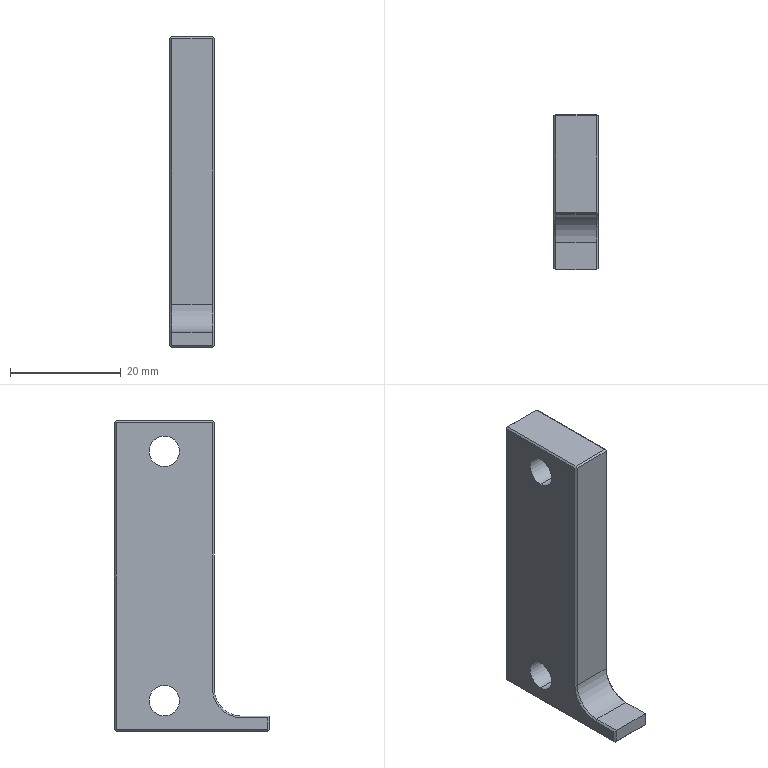Part | NX | 1 solid | 31 faces | box 8 x 28 x 56 mm | volume 7927 mm3 | plane 24 | cylinder 5 | cone 2 | commonest cylinder face diameters 5.5 x4 10 x1
STEP:
#1=CARTESIAN_POINT('',(2319.8,254.1,-75.2));
#2=VERTEX_POINT('',#1);
#3=CARTESIAN_POINT('',(2327.2,254.1,-75.2));
#4=VERTEX_POINT('',#3);
#5=CARTESIAN_POINT('',(2323.5,254.1,-75.2));
#6=DIRECTION('',(1.,0.,0.));
#7=VECTOR('',#6,1000.);
#8=LINE('',#5,#7);
#9=EDGE_CURVE('',#2,#4,#8,.T.);
#10=ORIENTED_EDGE('',*,*,#9,.T.);
#11=CARTESIAN_POINT('',(2327.2,226.7,-75.2));
#12=VERTEX_POINT('',#11);
#13=CARTESIAN_POINT('',(2327.2,240.4,-75.2));
#14=DIRECTION('',(0.,1.,0.));
#15=VECTOR('',#14,1000.);
#16=LINE('',#13,#15);
#17=EDGE_CURVE('',#12,#4,#16,.T.);
#18=ORIENTED_EDGE('',*,*,#17,.F.);
#19=CARTESIAN_POINT('',(2319.8,226.7,-75.2));
#20=VERTEX_POINT('',#19);
#21=CARTESIAN_POINT('',(2323.5,226.7,-75.2));
#22=DIRECTION('',(-1.,0.,0.));
#23=VECTOR('',#22,1000.);
#24=LINE('',#21,#23);
#25=EDGE_CURVE('',#12,#20,#24,.T.);
#26=ORIENTED_EDGE('',*,*,#25,.T.);
#27=CARTESIAN_POINT('',(2319.8,240.4,-75.2));
#28=DIRECTION('',(0.,-1.,0.));
#29=VECTOR('',#28,1000.);
#30=LINE('',#27,#29);
#31=EDGE_CURVE('',#2,#20,#30,.T.);
#32=ORIENTED_EDGE('',*,*,#31,.F.);
#33=EDGE_LOOP('',(#10,#18,#26,#32));
#34=FACE_BOUND('',#33,.T.);
#35=CARTESIAN_POINT('',(2321.5,254.4,-75.2));
#36=DIRECTION('',(0.,0.,-1.));
#37=DIRECTION('',(-1.,0.,0.));
#38=AXIS2_PLACEMENT_3D('',#35,#36,#37);
#39=PLANE('',#38);
#40=ADVANCED_FACE('',(#34),#39,.T.);
#41=CARTESIAN_POINT('',(2319.8,254.4,-19.5));
#42=VERTEX_POINT('',#41);
#43=CARTESIAN_POINT('',(2327.2,254.4,-19.5));
#44=VERTEX_POINT('',#43);
#45=CARTESIAN_POINT('',(2323.5,254.4,-19.5));
#46=DIRECTION('',(1.,0.,0.));
#47=VECTOR('',#46,1000.);
#48=LINE('',#45,#47);
#49=EDGE_CURVE('',#42,#44,#48,.T.);
#50=ORIENTED_EDGE('',*,*,#49,.T.);
#51=CARTESIAN_POINT('',(2327.2,254.4,-74.9));
#52=VERTEX_POINT('',#51);
#53=CARTESIAN_POINT('',(2327.2,254.4,-47.2));
#54=DIRECTION('',(0.,0.,1.));
#55=VECTOR('',#54,1000.);
#56=LINE('',#53,#55);
#57=EDGE_CURVE('',#52,#44,#56,.T.);
#58=ORIENTED_EDGE('',*,*,#57,.F.);
#59=CARTESIAN_POINT('',(2319.8,254.4,-74.9));
#60=VERTEX_POINT('',#59);
#61=CARTESIAN_POINT('',(2323.5,254.4,-74.9));
#62=DIRECTION('',(1.,0.,0.));
#63=VECTOR('',#62,1000.);
#64=LINE('',#61,#63);
#65=EDGE_CURVE('',#60,#52,#64,.T.);
#66=ORIENTED_EDGE('',*,*,#65,.F.);
#67=CARTESIAN_POINT('',(2319.8,254.4,-47.2));
#68=DIRECTION('',(0.,0.,-1.));
#69=VECTOR('',#68,1000.);
#70=LINE('',#67,#69);
#71=EDGE_CURVE('',#42,#60,#70,.T.);
#72=ORIENTED_EDGE('',*,*,#71,.F.);
#73=EDGE_LOOP('',(#50,#58,#66,#72));
#74=FACE_BOUND('',#73,.T.);
#75=CARTESIAN_POINT('',(2321.5,254.4,-19.2));
#76=DIRECTION('',(0.,1.,0.));
#77=DIRECTION('',(1.,0.,0.));
#78=AXIS2_PLACEMENT_3D('',#75,#76,#77);
#79=PLANE('',#78);
#80=ADVANCED_FACE('',(#74),#79,.T.);
#81=CARTESIAN_POINT('',(2319.8,236.7,-19.2));
#82=VERTEX_POINT('',#81);
#83=CARTESIAN_POINT('',(2327.2,236.7,-19.2));
#84=VERTEX_POINT('',#83);
#85=CARTESIAN_POINT('',(2323.5,236.7,-19.2));
#86=DIRECTION('',(1.,0.,0.));
#87=VECTOR('',#86,1000.);
#88=LINE('',#85,#87);
#89=EDGE_CURVE('',#82,#84,#88,.T.);
#90=ORIENTED_EDGE('',*,*,#89,.T.);
#91=CARTESIAN_POINT('',(2327.2,254.1,-19.2));
#92=VERTEX_POINT('',#91);
#93=CARTESIAN_POINT('',(2327.2,245.4,-19.2));
#94=DIRECTION('',(0.,-1.,0.));
#95=VECTOR('',#94,1000.);
#96=LINE('',#93,#95);
#97=EDGE_CURVE('',#92,#84,#96,.T.);
#98=ORIENTED_EDGE('',*,*,#97,.F.);
#99=CARTESIAN_POINT('',(2319.8,254.1,-19.2));
#100=VERTEX_POINT('',#99);
#101=CARTESIAN_POINT('',(2323.5,254.1,-19.2));
#102=DIRECTION('',(1.,0.,0.));
#103=VECTOR('',#102,1000.);
#104=LINE('',#101,#103);
#105=EDGE_CURVE('',#100,#92,#104,.T.);
#106=ORIENTED_EDGE('',*,*,#105,.F.);
#107=CARTESIAN_POINT('',(2319.8,245.4,-19.2));
#108=DIRECTION('',(0.,1.,0.));
#109=VECTOR('',#108,1000.);
#110=LINE('',#107,#109);
#111=EDGE_CURVE('',#82,#100,#110,.T.);
#112=ORIENTED_EDGE('',*,*,#111,.F.);
#113=EDGE_LOOP('',(#90,#98,#106,#112));
#114=FACE_BOUND('',#113,.T.);
#115=CARTESIAN_POINT('',(2321.5,236.4,-19.2));
#116=DIRECTION('',(0.,0.,1.));
#117=DIRECTION('',(1.,0.,0.));
#118=AXIS2_PLACEMENT_3D('',#115,#116,#117);
#119=PLANE('',#118);
#120=ADVANCED_FACE('',(#114),#119,.T.);
#121=CARTESIAN_POINT('',(2327.2,236.4,-67.5));
#122=VERTEX_POINT('',#121);
#123=CARTESIAN_POINT('',(2319.8,236.4,-67.5));
#124=VERTEX_POINT('',#123);
#125=CARTESIAN_POINT('',(2321.5,236.4,-67.5));
#126=DIRECTION('',(-1.,0.,0.));
#127=VECTOR('',#126,1000.);
#128=LINE('',#125,#127);
#129=EDGE_CURVE('',#122,#124,#128,.T.);
#130=ORIENTED_EDGE('',*,*,#129,.F.);
#131=CARTESIAN_POINT('',(2327.2,236.4,-19.5));
#132=VERTEX_POINT('',#131);
#133=CARTESIAN_POINT('',(2327.2,236.4,-43.35));
#134=DIRECTION('',(0.,0.,-1.));
#135=VECTOR('',#134,1000.);
#136=LINE('',#133,#135);
#137=EDGE_CURVE('',#132,#122,#136,.T.);
#138=ORIENTED_EDGE('',*,*,#137,.F.);
#139=CARTESIAN_POINT('',(2319.8,236.4,-19.5));
#140=VERTEX_POINT('',#139);
#141=CARTESIAN_POINT('',(2323.5,236.4,-19.5));
#142=DIRECTION('',(1.,0.,0.));
#143=VECTOR('',#142,1000.);
#144=LINE('',#141,#143);
#145=EDGE_CURVE('',#140,#132,#144,.T.);
#146=ORIENTED_EDGE('',*,*,#145,.F.);
#147=CARTESIAN_POINT('',(2319.8,236.4,-43.35));
#148=DIRECTION('',(0.,0.,1.));
#149=VECTOR('',#148,1000.);
#150=LINE('',#147,#149);
#151=EDGE_CURVE('',#124,#140,#150,.T.);
#152=ORIENTED_EDGE('',*,*,#151,.F.);
#153=EDGE_LOOP('',(#130,#138,#146,#152));
#154=FACE_BOUND('',#153,.T.);
#155=CARTESIAN_POINT('',(2321.5,236.4,-75.2));
#156=DIRECTION('',(0.,-1.,0.));
#157=DIRECTION('',(0.,0.,-1.));
#158=AXIS2_PLACEMENT_3D('',#155,#156,#157);
#159=PLANE('',#158);
#160=ADVANCED_FACE('',(#154),#159,.T.);
#161=CARTESIAN_POINT('',(2319.8,226.4,-72.5));
#162=VERTEX_POINT('',#161);
#163=CARTESIAN_POINT('',(2319.8,226.4,-74.9));
#164=VERTEX_POINT('',#163);
#165=CARTESIAN_POINT('',(2319.8,226.4,-73.85));
#166=DIRECTION('',(0.,0.,-1.));
#167=VECTOR('',#166,1000.);
#168=LINE('',#165,#167);
#169=EDGE_CURVE('',#162,#164,#168,.T.);
#170=ORIENTED_EDGE('',*,*,#169,.T.);
#171=CARTESIAN_POINT('',(2327.2,226.4,-74.9));
#172=VERTEX_POINT('',#171);
#173=CARTESIAN_POINT('',(2323.5,226.4,-74.9));
#174=DIRECTION('',(-1.,0.,0.));
#175=VECTOR('',#174,1000.);
#176=LINE('',#173,#175);
#177=EDGE_CURVE('',#172,#164,#176,.T.);
#178=ORIENTED_EDGE('',*,*,#177,.F.);
#179=CARTESIAN_POINT('',(2327.2,226.4,-72.5));
#180=VERTEX_POINT('',#179);
#181=CARTESIAN_POINT('',(2327.2,226.4,-73.85));
#182=DIRECTION('',(0.,0.,-1.));
#183=VECTOR('',#182,1000.);
#184=LINE('',#181,#183);
#185=EDGE_CURVE('',#180,#172,#184,.T.);
#186=ORIENTED_EDGE('',*,*,#185,.F.);
#187=CARTESIAN_POINT('',(2321.5,226.4,-72.5));
#188=DIRECTION('',(-1.,0.,0.));
#189=VECTOR('',#188,1000.);
#190=LINE('',#187,#189);
#191=EDGE_CURVE('',#180,#162,#190,.T.);
#192=ORIENTED_EDGE('',*,*,#191,.T.);
#193=EDGE_LOOP('',(#170,#178,#186,#192));
#194=FACE_BOUND('',#193,.T.);
#195=CARTESIAN_POINT('',(2325.077,226.4,-68.526));
#196=DIRECTION('',(0.,-1.,0.));
#197=DIRECTION('',(0.,0.,-1.));
#198=AXIS2_PLACEMENT_3D('',#195,#196,#197);
#199=PLANE('',#198);
#200=ADVANCED_FACE('',(#194),#199,.T.);
#201=CARTESIAN_POINT('',(2319.8,231.4,-72.5));
#202=VERTEX_POINT('',#201);
#203=CARTESIAN_POINT('',(2319.8,228.9,-72.5));
#204=DIRECTION('',(0.,-1.,0.));
#205=VECTOR('',#204,1000.);
#206=LINE('',#203,#205);
#207=EDGE_CURVE('',#202,#162,#206,.T.);
#208=ORIENTED_EDGE('',*,*,#207,.T.);
#209=ORIENTED_EDGE('',*,*,#191,.F.);
#210=CARTESIAN_POINT('',(2327.2,231.4,-72.5));
#211=VERTEX_POINT('',#210);
#212=CARTESIAN_POINT('',(2327.2,228.9,-72.5));
#213=DIRECTION('',(0.,-1.,0.));
#214=VECTOR('',#213,1000.);
#215=LINE('',#212,#214);
#216=EDGE_CURVE('',#211,#180,#215,.T.);
#217=ORIENTED_EDGE('',*,*,#216,.F.);
#218=CARTESIAN_POINT('',(2321.5,231.4,-72.5));
#219=DIRECTION('',(-1.,0.,0.));
#220=VECTOR('',#219,1000.);
#221=LINE('',#218,#220);
#222=EDGE_CURVE('',#211,#202,#221,.T.);
#223=ORIENTED_EDGE('',*,*,#222,.T.);
#224=EDGE_LOOP('',(#208,#209,#217,#223));
#225=FACE_BOUND('',#224,.T.);
#226=CARTESIAN_POINT('',(2321.5,236.4,-72.5));
#227=DIRECTION('',(0.,0.,1.));
#228=DIRECTION('',(1.,0.,0.));
#229=AXIS2_PLACEMENT_3D('',#226,#227,#228);
#230=PLANE('',#229);
#231=ADVANCED_FACE('',(#225),#230,.T.);
#232=CARTESIAN_POINT('',(2327.2,231.4,-67.5));
#233=DIRECTION('',(-1.,0.,0.));
#234=DIRECTION('',(0.,0.,-1.));
#235=AXIS2_PLACEMENT_3D('',#232,#233,#234);
#236=CIRCLE('',#235,5.);
#237=EDGE_CURVE('',#122,#211,#236,.T.);
#238=ORIENTED_EDGE('',*,*,#237,.F.);
#239=ORIENTED_EDGE('',*,*,#129,.T.);
#240=CARTESIAN_POINT('',(2319.8,231.4,-67.5));
#241=DIRECTION('',(-1.,0.,0.));
#242=DIRECTION('',(0.,0.,-1.));
#243=AXIS2_PLACEMENT_3D('',#240,#241,#242);
#244=CIRCLE('',#243,5.);
#245=EDGE_CURVE('',#124,#202,#244,.T.);
#246=ORIENTED_EDGE('',*,*,#245,.T.);
#247=ORIENTED_EDGE('',*,*,#222,.F.);
#248=EDGE_LOOP('',(#238,#239,#246,#247));
#249=FACE_BOUND('',#248,.T.);
#250=CARTESIAN_POINT('',(2321.5,231.4,-67.5));
#251=DIRECTION('',(-1.,0.,0.));
#252=DIRECTION('',(0.,0.,-1.));
#253=AXIS2_PLACEMENT_3D('',#250,#251,#252);
#254=CYLINDRICAL_SURFACE('',#253,5.);
#255=ADVANCED_FACE('',(#249),#254,.F.);
#256=ORIENTED_EDGE('',*,*,#9,.F.);
#257=CARTESIAN_POINT('',(2319.65,254.25,-75.05));
#258=VERTEX_POINT('',#257);
#259=CARTESIAN_POINT('',(2327.326,246.574,-82.726));
#260=DIRECTION('',(0.5774,-0.5774,-0.5774));
#261=VECTOR('',#260,1000.);
#262=LINE('',#259,#261);
#263=EDGE_CURVE('',#258,#2,#262,.T.);
#264=ORIENTED_EDGE('',*,*,#263,.F.);
#265=CARTESIAN_POINT('',(2321.5,256.1,-73.2));
#266=DIRECTION('',(0.5774,0.5774,0.5774));
#267=VECTOR('',#266,1000.);
#268=LINE('',#265,#267);
#269=EDGE_CURVE('',#258,#60,#268,.T.);
#270=ORIENTED_EDGE('',*,*,#269,.T.);
#271=ORIENTED_EDGE('',*,*,#65,.T.);
#272=CARTESIAN_POINT('',(2327.35,254.25,-75.05));
#273=VERTEX_POINT('',#272);
#274=CARTESIAN_POINT('',(2321.5,260.1,-69.2));
#275=DIRECTION('',(0.5774,-0.5774,-0.5774));
#276=VECTOR('',#275,1000.);
#277=LINE('',#274,#276);
#278=EDGE_CURVE('',#52,#273,#277,.T.);
#279=ORIENTED_EDGE('',*,*,#278,.T.);
#280=CARTESIAN_POINT('',(2319.674,246.574,-82.726));
#281=DIRECTION('',(-0.5774,-0.5774,-0.5774));
#282=VECTOR('',#281,1000.);
#283=LINE('',#280,#282);
#284=EDGE_CURVE('',#273,#4,#283,.T.);
#285=ORIENTED_EDGE('',*,*,#284,.T.);
#286=EDGE_LOOP('',(#256,#264,#270,#271,#279,#285));
#287=FACE_BOUND('',#286,.T.);
#288=CARTESIAN_POINT('',(2323.5,254.25,-75.05));
#289=DIRECTION('',(0.,0.7071,-0.7071));
#290=DIRECTION('',(-1.,0.,0.));
#291=AXIS2_PLACEMENT_3D('',#288,#289,#290);
#292=PLANE('',#291);
#293=ADVANCED_FACE('',(#287),#292,.T.);
#294=ORIENTED_EDGE('',*,*,#49,.F.);
#295=CARTESIAN_POINT('',(2319.65,254.25,-19.35));
#296=VERTEX_POINT('',#295);
#297=CARTESIAN_POINT('',(2345.565,280.165,-45.265));
#298=DIRECTION('',(0.5774,0.5774,-0.5774));
#299=VECTOR('',#298,1000.);
#300=LINE('',#297,#299);
#301=EDGE_CURVE('',#296,#42,#300,.T.);
#302=ORIENTED_EDGE('',*,*,#301,.F.);
#303=CARTESIAN_POINT('',(2293.735,280.165,-45.265));
#304=DIRECTION('',(0.5774,-0.5774,0.5774));
#305=VECTOR('',#304,1000.);
#306=LINE('',#303,#305);
#307=EDGE_CURVE('',#296,#100,#306,.T.);
#308=ORIENTED_EDGE('',*,*,#307,.T.);
#309=ORIENTED_EDGE('',*,*,#105,.T.);
#310=CARTESIAN_POINT('',(2327.35,254.25,-19.35));
#311=VERTEX_POINT('',#310);
#312=CARTESIAN_POINT('',(2353.265,280.165,-45.265));
#313=DIRECTION('',(0.5774,0.5774,-0.5774));
#314=VECTOR('',#313,1000.);
#315=LINE('',#312,#314);
#316=EDGE_CURVE('',#92,#311,#315,.T.);
#317=ORIENTED_EDGE('',*,*,#316,.T.);
#318=CARTESIAN_POINT('',(2301.435,280.165,-45.265));
#319=DIRECTION('',(0.5774,-0.5774,0.5774));
#320=VECTOR('',#319,1000.);
#321=LINE('',#318,#320);
#322=EDGE_CURVE('',#44,#311,#321,.T.);
#323=ORIENTED_EDGE('',*,*,#322,.F.);
#324=EDGE_LOOP('',(#294,#302,#308,#309,#317,#323));
#325=FACE_BOUND('',#324,.T.);
#326=CARTESIAN_POINT('',(2323.5,254.25,-19.35));
#327=DIRECTION('',(0.,0.7071,0.7071));
#328=DIRECTION('',(1.,0.,0.));
#329=AXIS2_PLACEMENT_3D('',#326,#327,#328);
#330=PLANE('',#329);
#331=ADVANCED_FACE('',(#325),#330,.T.);
#332=ORIENTED_EDGE('',*,*,#89,.F.);
#333=CARTESIAN_POINT('',(2319.65,236.55,-19.35));
#334=VERTEX_POINT('',#333);
#335=CARTESIAN_POINT('',(2293.735,210.635,-45.265));
#336=DIRECTION('',(0.5774,0.5774,0.5774));
#337=VECTOR('',#336,1000.);
#338=LINE('',#335,#337);
#339=EDGE_CURVE('',#334,#82,#338,.T.);
#340=ORIENTED_EDGE('',*,*,#339,.F.);
#341=CARTESIAN_POINT('',(2345.565,210.635,-45.265));
#342=DIRECTION('',(0.5774,-0.5774,-0.5774));
#343=VECTOR('',#342,1000.);
#344=LINE('',#341,#343);
#345=EDGE_CURVE('',#334,#140,#344,.T.);
#346=ORIENTED_EDGE('',*,*,#345,.T.);
#347=ORIENTED_EDGE('',*,*,#145,.T.);
#348=CARTESIAN_POINT('',(2327.35,236.55,-19.35));
#349=VERTEX_POINT('',#348);
#350=CARTESIAN_POINT('',(2301.435,210.635,-45.265));
#351=DIRECTION('',(0.5774,0.5774,0.5774));
#352=VECTOR('',#351,1000.);
#353=LINE('',#350,#352);
#354=EDGE_CURVE('',#132,#349,#353,.T.);
#355=ORIENTED_EDGE('',*,*,#354,.T.);
#356=CARTESIAN_POINT('',(2353.265,210.635,-45.265));
#357=DIRECTION('',(-0.5774,0.5774,0.5774));
#358=VECTOR('',#357,1000.);
#359=LINE('',#356,#358);
#360=EDGE_CURVE('',#349,#84,#359,.T.);
#361=ORIENTED_EDGE('',*,*,#360,.T.);
#362=EDGE_LOOP('',(#332,#340,#346,#347,#355,#361));
#363=FACE_BOUND('',#362,.T.);
#364=CARTESIAN_POINT('',(2323.5,236.55,-19.35));
#365=DIRECTION('',(0.,-0.7071,0.7071));
#366=DIRECTION('',(-1.,0.,0.));
#367=AXIS2_PLACEMENT_3D('',#364,#365,#366);
#368=PLANE('',#367);
#369=ADVANCED_FACE('',(#363),#368,.T.);
#370=ORIENTED_EDGE('',*,*,#245,.F.);
#371=CARTESIAN_POINT('',(2319.5,236.7,-67.5));
#372=VERTEX_POINT('',#371);
#373=CARTESIAN_POINT('',(2319.8,236.4,-67.5));
#374=DIRECTION('',(-0.7071,0.7071,0.));
#375=VECTOR('',#374,1000.);
#376=LINE('',#373,#375);
#377=EDGE_CURVE('',#124,#372,#376,.T.);
#378=ORIENTED_EDGE('',*,*,#377,.T.);
#379=CARTESIAN_POINT('',(2319.5,231.4,-72.8));
#380=VERTEX_POINT('',#379);
#381=CARTESIAN_POINT('',(2319.5,231.4,-67.5));
#382=DIRECTION('',(-1.,0.,0.));
#383=DIRECTION('',(0.,0.,-1.));
#384=AXIS2_PLACEMENT_3D('',#381,#382,#383);
#385=CIRCLE('',#384,5.3);
#386=EDGE_CURVE('',#372,#380,#385,.T.);
#387=ORIENTED_EDGE('',*,*,#386,.T.);
#388=CARTESIAN_POINT('',(2319.5,231.4,-72.8));
#389=DIRECTION('',(0.7071,0.,0.7071));
#390=VECTOR('',#389,1000.);
#391=LINE('',#388,#390);
#392=EDGE_CURVE('',#380,#202,#391,.T.);
#393=ORIENTED_EDGE('',*,*,#392,.T.);
#394=EDGE_LOOP('',(#370,#378,#387,#393));
#395=FACE_BOUND('',#394,.T.);
#396=CARTESIAN_POINT('',(2319.8,231.4,-67.5));
#397=DIRECTION('',(-1.,0.,0.));
#398=DIRECTION('',(0.,1.,0.));
#399=AXIS2_PLACEMENT_3D('',#396,#397,#398);
#400=CONICAL_SURFACE('',#399,5.,0.7854);
#401=ADVANCED_FACE('',(#395),#400,.F.);
#402=ORIENTED_EDGE('',*,*,#207,.F.);
#403=ORIENTED_EDGE('',*,*,#392,.F.);
#404=CARTESIAN_POINT('',(2319.5,226.7,-72.8));
#405=VERTEX_POINT('',#404);
#406=CARTESIAN_POINT('',(2319.5,228.9,-72.8));
#407=DIRECTION('',(0.,-1.,0.));
#408=VECTOR('',#407,1000.);
#409=LINE('',#406,#408);
#410=EDGE_CURVE('',#380,#405,#409,.T.);
#411=ORIENTED_EDGE('',*,*,#410,.T.);
#412=CARTESIAN_POINT('',(2299.626,246.574,-92.674));
#413=DIRECTION('',(-0.5774,0.5774,-0.5774));
#414=VECTOR('',#413,1000.);
#415=LINE('',#412,#414);
#416=EDGE_CURVE('',#162,#405,#415,.T.);
#417=ORIENTED_EDGE('',*,*,#416,.F.);
#418=EDGE_LOOP('',(#402,#403,#411,#417));
#419=FACE_BOUND('',#418,.T.);
#420=CARTESIAN_POINT('',(2319.65,228.9,-72.65));
#421=DIRECTION('',(-0.7071,0.,0.7071));
#422=DIRECTION('',(0.,1.,0.));
#423=AXIS2_PLACEMENT_3D('',#420,#421,#422);
#424=PLANE('',#423);
#425=ADVANCED_FACE('',(#419),#424,.T.);
#426=ORIENTED_EDGE('',*,*,#237,.T.);
#427=CARTESIAN_POINT('',(2327.5,231.4,-72.8));
#428=VERTEX_POINT('',#427);
#429=CARTESIAN_POINT('',(2327.2,231.4,-72.5));
#430=DIRECTION('',(0.7071,0.,-0.7071));
#431=VECTOR('',#430,1000.);
#432=LINE('',#429,#431);
#433=EDGE_CURVE('',#211,#428,#432,.T.);
#434=ORIENTED_EDGE('',*,*,#433,.T.);
#435=CARTESIAN_POINT('',(2327.5,236.7,-67.5));
#436=VERTEX_POINT('',#435);
#437=CARTESIAN_POINT('',(2327.5,231.4,-67.5));
#438=DIRECTION('',(-1.,0.,0.));
#439=DIRECTION('',(0.,0.,-1.));
#440=AXIS2_PLACEMENT_3D('',#437,#438,#439);
#441=CIRCLE('',#440,5.3);
#442=EDGE_CURVE('',#436,#428,#441,.T.);
#443=ORIENTED_EDGE('',*,*,#442,.F.);
#444=CARTESIAN_POINT('',(2327.2,236.4,-67.5));
#445=DIRECTION('',(0.7071,0.7071,0.));
#446=VECTOR('',#445,1000.);
#447=LINE('',#444,#446);
#448=EDGE_CURVE('',#122,#436,#447,.T.);
#449=ORIENTED_EDGE('',*,*,#448,.F.);
#450=EDGE_LOOP('',(#426,#434,#443,#449));
#451=FACE_BOUND('',#450,.T.);
#452=CARTESIAN_POINT('',(2327.2,231.4,-67.5));
#453=DIRECTION('',(1.,0.,0.));
#454=DIRECTION('',(0.,-1.,0.));
#455=AXIS2_PLACEMENT_3D('',#452,#453,#454);
#456=CONICAL_SURFACE('',#455,5.,0.7854);
#457=ADVANCED_FACE('',(#451),#456,.F.);
#458=ORIENTED_EDGE('',*,*,#177,.T.);
#459=CARTESIAN_POINT('',(2319.65,226.55,-75.05));
#460=VERTEX_POINT('',#459);
#461=CARTESIAN_POINT('',(2349.435,196.765,-45.265));
#462=DIRECTION('',(-0.5774,0.5774,-0.5774));
#463=VECTOR('',#462,1000.);
#464=LINE('',#461,#463);
#465=EDGE_CURVE('',#164,#460,#464,.T.);
#466=ORIENTED_EDGE('',*,*,#465,.T.);
#467=CARTESIAN_POINT('',(2289.865,196.765,-45.265));
#468=DIRECTION('',(0.5774,0.5774,-0.5774));
#469=VECTOR('',#468,1000.);
#470=LINE('',#467,#469);
#471=EDGE_CURVE('',#460,#20,#470,.T.);
#472=ORIENTED_EDGE('',*,*,#471,.T.);
#473=ORIENTED_EDGE('',*,*,#25,.F.);
#474=CARTESIAN_POINT('',(2327.35,226.55,-75.05));
#475=VERTEX_POINT('',#474);
#476=CARTESIAN_POINT('',(2357.135,196.765,-45.265));
#477=DIRECTION('',(0.5774,-0.5774,0.5774));
#478=VECTOR('',#477,1000.);
#479=LINE('',#476,#478);
#480=EDGE_CURVE('',#12,#475,#479,.T.);
#481=ORIENTED_EDGE('',*,*,#480,.T.);
#482=CARTESIAN_POINT('',(2297.565,196.765,-45.265));
#483=DIRECTION('',(0.5774,0.5774,-0.5774));
#484=VECTOR('',#483,1000.);
#485=LINE('',#482,#484);
#486=EDGE_CURVE('',#172,#475,#485,.T.);
#487=ORIENTED_EDGE('',*,*,#486,.F.);
#488=EDGE_LOOP('',(#458,#466,#472,#473,#481,#487));
#489=FACE_BOUND('',#488,.T.);
#490=CARTESIAN_POINT('',(2323.5,226.55,-75.05));
#491=DIRECTION('',(0.,0.7071,0.7071));
#492=DIRECTION('',(1.,0.,0.));
#493=AXIS2_PLACEMENT_3D('',#490,#491,#492);
#494=PLANE('',#493);
#495=ADVANCED_FACE('',(#489),#494,.F.);
#496=ORIENTED_EDGE('',*,*,#185,.T.);
#497=ORIENTED_EDGE('',*,*,#486,.T.);
#498=CARTESIAN_POINT('',(2327.5,226.7,-74.9));
#499=VERTEX_POINT('',#498);
#500=CARTESIAN_POINT('',(2357.135,256.335,-45.265));
#501=DIRECTION('',(-0.5774,-0.5774,-0.5774));
#502=VECTOR('',#501,1000.);
#503=LINE('',#500,#502);
#504=EDGE_CURVE('',#499,#475,#503,.T.);
#505=ORIENTED_EDGE('',*,*,#504,.F.);
#506=CARTESIAN_POINT('',(2327.5,226.7,-72.8));
#507=VERTEX_POINT('',#506);
#508=CARTESIAN_POINT('',(2327.5,226.7,-73.85));
#509=DIRECTION('',(0.,0.,-1.));
#510=VECTOR('',#509,1000.);
#511=LINE('',#508,#510);
#512=EDGE_CURVE('',#507,#499,#511,.T.);
#513=ORIENTED_EDGE('',*,*,#512,.F.);
#514=CARTESIAN_POINT('',(2299.965,199.165,-45.265));
#515=DIRECTION('',(0.5774,0.5774,-0.5774));
#516=VECTOR('',#515,1000.);
#517=LINE('',#514,#516);
#518=EDGE_CURVE('',#180,#507,#517,.T.);
#519=ORIENTED_EDGE('',*,*,#518,.F.);
#520=EDGE_LOOP('',(#496,#497,#505,#513,#519));
#521=FACE_BOUND('',#520,.T.);
#522=CARTESIAN_POINT('',(2327.35,226.55,-73.85));
#523=DIRECTION('',(-0.7071,0.7071,0.));
#524=DIRECTION('',(0.,0.,1.));
#525=AXIS2_PLACEMENT_3D('',#522,#523,#524);
#526=PLANE('',#525);
#527=ADVANCED_FACE('',(#521),#526,.F.);
#528=ORIENTED_EDGE('',*,*,#169,.F.);
#529=ORIENTED_EDGE('',*,*,#416,.T.);
#530=CARTESIAN_POINT('',(2319.5,226.7,-74.9));
#531=VERTEX_POINT('',#530);
#532=CARTESIAN_POINT('',(2319.5,226.7,-73.85));
#533=DIRECTION('',(0.,0.,-1.));
#534=VECTOR('',#533,1000.);
#535=LINE('',#532,#534);
#536=EDGE_CURVE('',#405,#531,#535,.T.);
#537=ORIENTED_EDGE('',*,*,#536,.T.);
#538=CARTESIAN_POINT('',(2299.626,246.574,-55.026));
#539=DIRECTION('',(0.5774,-0.5774,-0.5774));
#540=VECTOR('',#539,1000.);
#541=LINE('',#538,#540);
#542=EDGE_CURVE('',#531,#460,#541,.T.);
#543=ORIENTED_EDGE('',*,*,#542,.T.);
#544=ORIENTED_EDGE('',*,*,#465,.F.);
#545=EDGE_LOOP('',(#528,#529,#537,#543,#544));
#546=FACE_BOUND('',#545,.T.);
#547=CARTESIAN_POINT('',(2319.65,226.55,-73.85));
#548=DIRECTION('',(-0.7071,-0.7071,0.));
#549=DIRECTION('',(-0.7071,0.7071,0.));
#550=AXIS2_PLACEMENT_3D('',#547,#548,#549);
#551=PLANE('',#550);
#552=ADVANCED_FACE('',(#546),#551,.T.);
#553=CARTESIAN_POINT('',(2327.5,228.9,-72.8));
#554=DIRECTION('',(0.,-1.,0.));
#555=VECTOR('',#554,1000.);
#556=LINE('',#553,#555);
#557=EDGE_CURVE('',#428,#507,#556,.T.);
#558=ORIENTED_EDGE('',*,*,#557,.T.);
#559=ORIENTED_EDGE('',*,*,#512,.T.);
#560=CARTESIAN_POINT('',(2327.5,254.1,-74.9));
#561=VERTEX_POINT('',#560);
#562=CARTESIAN_POINT('',(2327.5,240.4,-74.9));
#563=DIRECTION('',(0.,1.,0.));
#564=VECTOR('',#563,1000.);
#565=LINE('',#562,#564);
#566=EDGE_CURVE('',#499,#561,#565,.T.);
#567=ORIENTED_EDGE('',*,*,#566,.T.);
#568=CARTESIAN_POINT('',(2327.5,254.1,-19.5));
#569=VERTEX_POINT('',#568);
#570=CARTESIAN_POINT('',(2327.5,254.1,-47.2));
#571=DIRECTION('',(0.,0.,1.));
#572=VECTOR('',#571,1000.);
#573=LINE('',#570,#572);
#574=EDGE_CURVE('',#561,#569,#573,.T.);
#575=ORIENTED_EDGE('',*,*,#574,.T.);
#576=CARTESIAN_POINT('',(2327.5,236.7,-19.5));
#577=VERTEX_POINT('',#576);
#578=CARTESIAN_POINT('',(2327.5,245.4,-19.5));
#579=DIRECTION('',(0.,-1.,0.));
#580=VECTOR('',#579,1000.);
#581=LINE('',#578,#580);
#582=EDGE_CURVE('',#569,#577,#581,.T.);
#583=ORIENTED_EDGE('',*,*,#582,.T.);
#584=CARTESIAN_POINT('',(2327.5,236.7,-43.35));
#585=DIRECTION('',(0.,0.,-1.));
#586=VECTOR('',#585,1000.);
#587=LINE('',#584,#586);
#588=EDGE_CURVE('',#577,#436,#587,.T.);
#589=ORIENTED_EDGE('',*,*,#588,.T.);
#590=ORIENTED_EDGE('',*,*,#442,.T.);
#591=EDGE_LOOP('',(#558,#559,#567,#575,#583,#589,#590));
#592=FACE_BOUND('',#591,.T.);
#593=CARTESIAN_POINT('',(2327.5,245.4,-72.45));
#594=VERTEX_POINT('',#593);
#595=CARTESIAN_POINT('',(2327.5,245.4,-66.95));
#596=VERTEX_POINT('',#595);
#597=CARTESIAN_POINT('',(2327.5,245.4,-69.7));
#598=DIRECTION('',(1.,0.,0.));
#599=DIRECTION('',(0.,0.,-1.));
#600=AXIS2_PLACEMENT_3D('',#597,#598,#599);
#601=CIRCLE('',#600,2.75);
#602=EDGE_CURVE('',#594,#596,#601,.T.);
#603=ORIENTED_EDGE('',*,*,#602,.F.);
#604=CARTESIAN_POINT('',(2327.5,245.4,-69.7));
#605=DIRECTION('',(1.,0.,0.));
#606=DIRECTION('',(0.,0.,-1.));
#607=AXIS2_PLACEMENT_3D('',#604,#605,#606);
#608=CIRCLE('',#607,2.75);
#609=EDGE_CURVE('',#596,#594,#608,.T.);
#610=ORIENTED_EDGE('',*,*,#609,.F.);
#611=EDGE_LOOP('',(#603,#610));
#612=FACE_BOUND('',#611,.T.);
#613=CARTESIAN_POINT('',(2327.5,245.4,-21.95));
#614=VERTEX_POINT('',#613);
#615=CARTESIAN_POINT('',(2327.5,245.4,-27.45));
#616=VERTEX_POINT('',#615);
#617=CARTESIAN_POINT('',(2327.5,245.4,-24.7));
#618=DIRECTION('',(1.,0.,0.));
#619=DIRECTION('',(0.,0.,-1.));
#620=AXIS2_PLACEMENT_3D('',#617,#618,#619);
#621=CIRCLE('',#620,2.75);
#622=EDGE_CURVE('',#614,#616,#621,.T.);
#623=ORIENTED_EDGE('',*,*,#622,.F.);
#624=CARTESIAN_POINT('',(2327.5,245.4,-24.7));
#625=DIRECTION('',(1.,0.,0.));
#626=DIRECTION('',(0.,0.,-1.));
#627=AXIS2_PLACEMENT_3D('',#624,#625,#626);
#628=CIRCLE('',#627,2.75);
#629=EDGE_CURVE('',#616,#614,#628,.T.);
#630=ORIENTED_EDGE('',*,*,#629,.F.);
#631=EDGE_LOOP('',(#623,#630));
#632=FACE_BOUND('',#631,.T.);
#633=CARTESIAN_POINT('',(2327.5,246.574,-45.265));
#634=DIRECTION('',(1.,0.,0.));
#635=DIRECTION('',(0.,1.,0.));
#636=AXIS2_PLACEMENT_3D('',#633,#634,#635);
#637=PLANE('',#636);
#638=ADVANCED_FACE('',(#592,#612,#632),#637,.T.);
#639=CARTESIAN_POINT('',(2319.5,245.4,-27.45));
#640=VERTEX_POINT('',#639);
#641=CARTESIAN_POINT('',(2319.5,245.4,-21.95));
#642=VERTEX_POINT('',#641);
#643=CARTESIAN_POINT('',(2319.5,245.4,-24.7));
#644=DIRECTION('',(1.,0.,0.));
#645=DIRECTION('',(0.,0.,-1.));
#646=AXIS2_PLACEMENT_3D('',#643,#644,#645);
#647=CIRCLE('',#646,2.75);
#648=EDGE_CURVE('',#640,#642,#647,.T.);
#649=ORIENTED_EDGE('',*,*,#648,.F.);
#650=CARTESIAN_POINT('',(2320.9,245.4,-27.45));
#651=DIRECTION('',(1.,0.,0.));
#652=VECTOR('',#651,1000.);
#653=LINE('',#650,#652);
#654=EDGE_CURVE('',#616,#640,#653,.F.);
#655=ORIENTED_EDGE('',*,*,#654,.F.);
#656=ORIENTED_EDGE('',*,*,#629,.T.);
#657=CARTESIAN_POINT('',(2320.9,245.4,-21.95));
#658=DIRECTION('',(1.,0.,0.));
#659=VECTOR('',#658,1000.);
#660=LINE('',#657,#659);
#661=EDGE_CURVE('',#614,#642,#660,.F.);
#662=ORIENTED_EDGE('',*,*,#661,.T.);
#663=EDGE_LOOP('',(#649,#655,#656,#662));
#664=FACE_BOUND('',#663,.T.);
#665=CARTESIAN_POINT('',(2320.9,245.4,-24.7));
#666=DIRECTION('',(1.,0.,0.));
#667=DIRECTION('',(0.,0.,-1.));
#668=AXIS2_PLACEMENT_3D('',#665,#666,#667);
#669=CYLINDRICAL_SURFACE('',#668,2.75);
#670=ADVANCED_FACE('',(#664),#669,.F.);
#671=ORIENTED_EDGE('',*,*,#602,.T.);
#672=CARTESIAN_POINT('',(2319.5,245.4,-66.95));
#673=VERTEX_POINT('',#672);
#674=CARTESIAN_POINT('',(2320.9,245.4,-66.95));
#675=DIRECTION('',(1.,0.,0.));
#676=VECTOR('',#675,1000.);
#677=LINE('',#674,#676);
#678=EDGE_CURVE('',#596,#673,#677,.F.);
#679=ORIENTED_EDGE('',*,*,#678,.T.);
#680=CARTESIAN_POINT('',(2319.5,245.4,-72.45));
#681=VERTEX_POINT('',#680);
#682=CARTESIAN_POINT('',(2319.5,245.4,-69.7));
#683=DIRECTION('',(1.,0.,0.));
#684=DIRECTION('',(0.,0.,-1.));
#685=AXIS2_PLACEMENT_3D('',#682,#683,#684);
#686=CIRCLE('',#685,2.75);
#687=EDGE_CURVE('',#681,#673,#686,.T.);
#688=ORIENTED_EDGE('',*,*,#687,.F.);
#689=CARTESIAN_POINT('',(2320.9,245.4,-72.45));
#690=DIRECTION('',(1.,0.,0.));
#691=VECTOR('',#690,1000.);
#692=LINE('',#689,#691);
#693=EDGE_CURVE('',#594,#681,#692,.F.);
#694=ORIENTED_EDGE('',*,*,#693,.F.);
#695=EDGE_LOOP('',(#671,#679,#688,#694));
#696=FACE_BOUND('',#695,.T.);
#697=CARTESIAN_POINT('',(2320.9,245.4,-69.7));
#698=DIRECTION('',(1.,0.,0.));
#699=DIRECTION('',(0.,0.,-1.));
#700=AXIS2_PLACEMENT_3D('',#697,#698,#699);
#701=CYLINDRICAL_SURFACE('',#700,2.75);
#702=ADVANCED_FACE('',(#696),#701,.F.);
#703=ORIENTED_EDGE('',*,*,#566,.F.);
#704=ORIENTED_EDGE('',*,*,#504,.T.);
#705=ORIENTED_EDGE('',*,*,#480,.F.);
#706=ORIENTED_EDGE('',*,*,#17,.T.);
#707=ORIENTED_EDGE('',*,*,#284,.F.);
#708=CARTESIAN_POINT('',(2357.135,224.465,-45.265));
#709=DIRECTION('',(0.5774,-0.5774,0.5774));
#710=VECTOR('',#709,1000.);
#711=LINE('',#708,#710);
#712=EDGE_CURVE('',#273,#561,#711,.T.);
#713=ORIENTED_EDGE('',*,*,#712,.T.);
#714=EDGE_LOOP('',(#703,#704,#705,#706,#707,#713));
#715=FACE_BOUND('',#714,.T.);
#716=CARTESIAN_POINT('',(2327.35,240.4,-75.05));
#717=DIRECTION('',(0.7071,0.,-0.7071));
#718=DIRECTION('',(0.,-1.,0.));
#719=AXIS2_PLACEMENT_3D('',#716,#717,#718);
#720=PLANE('',#719);
#721=ADVANCED_FACE('',(#715),#720,.T.);
#722=ORIENTED_EDGE('',*,*,#574,.F.);
#723=ORIENTED_EDGE('',*,*,#712,.F.);
#724=ORIENTED_EDGE('',*,*,#278,.F.);
#725=ORIENTED_EDGE('',*,*,#57,.T.);
#726=ORIENTED_EDGE('',*,*,#322,.T.);
#727=CARTESIAN_POINT('',(2353.265,228.335,-45.265));
#728=DIRECTION('',(0.5774,-0.5774,-0.5774));
#729=VECTOR('',#728,1000.);
#730=LINE('',#727,#729);
#731=EDGE_CURVE('',#311,#569,#730,.T.);
#732=ORIENTED_EDGE('',*,*,#731,.T.);
#733=EDGE_LOOP('',(#722,#723,#724,#725,#726,#732));
#734=FACE_BOUND('',#733,.T.);
#735=CARTESIAN_POINT('',(2327.35,254.25,-47.2));
#736=DIRECTION('',(0.7071,0.7071,0.));
#737=DIRECTION('',(0.,0.,-1.));
#738=AXIS2_PLACEMENT_3D('',#735,#736,#737);
#739=PLANE('',#738);
#740=ADVANCED_FACE('',(#734),#739,.T.);
#741=ORIENTED_EDGE('',*,*,#582,.F.);
#742=ORIENTED_EDGE('',*,*,#731,.F.);
#743=ORIENTED_EDGE('',*,*,#316,.F.);
#744=ORIENTED_EDGE('',*,*,#97,.T.);
#745=ORIENTED_EDGE('',*,*,#360,.F.);
#746=CARTESIAN_POINT('',(2353.265,262.465,-45.265));
#747=DIRECTION('',(0.5774,0.5774,-0.5774));
#748=VECTOR('',#747,1000.);
#749=LINE('',#746,#748);
#750=EDGE_CURVE('',#349,#577,#749,.T.);
#751=ORIENTED_EDGE('',*,*,#750,.T.);
#752=EDGE_LOOP('',(#741,#742,#743,#744,#745,#751));
#753=FACE_BOUND('',#752,.T.);
#754=CARTESIAN_POINT('',(2327.35,245.4,-19.35));
#755=DIRECTION('',(0.7071,0.,0.7071));
#756=DIRECTION('',(0.,-1.,0.));
#757=AXIS2_PLACEMENT_3D('',#754,#755,#756);
#758=PLANE('',#757);
#759=ADVANCED_FACE('',(#753),#758,.T.);
#760=ORIENTED_EDGE('',*,*,#588,.F.);
#761=ORIENTED_EDGE('',*,*,#750,.F.);
#762=ORIENTED_EDGE('',*,*,#354,.F.);
#763=ORIENTED_EDGE('',*,*,#137,.T.);
#764=ORIENTED_EDGE('',*,*,#448,.T.);
#765=EDGE_LOOP('',(#760,#761,#762,#763,#764));
#766=FACE_BOUND('',#765,.T.);
#767=CARTESIAN_POINT('',(2327.35,236.55,-43.35));
#768=DIRECTION('',(0.7071,-0.7071,0.));
#769=DIRECTION('',(0.,0.,-1.));
#770=AXIS2_PLACEMENT_3D('',#767,#768,#769);
#771=PLANE('',#770);
#772=ADVANCED_FACE('',(#766),#771,.T.);
#773=ORIENTED_EDGE('',*,*,#557,.F.);
#774=ORIENTED_EDGE('',*,*,#433,.F.);
#775=ORIENTED_EDGE('',*,*,#216,.T.);
#776=ORIENTED_EDGE('',*,*,#518,.T.);
#777=EDGE_LOOP('',(#773,#774,#775,#776));
#778=FACE_BOUND('',#777,.T.);
#779=CARTESIAN_POINT('',(2327.35,228.9,-72.65));
#780=DIRECTION('',(0.7071,0.,0.7071));
#781=DIRECTION('',(0.,-1.,0.));
#782=AXIS2_PLACEMENT_3D('',#779,#780,#781);
#783=PLANE('',#782);
#784=ADVANCED_FACE('',(#778),#783,.T.);
#785=CARTESIAN_POINT('',(2319.5,236.7,-19.5));
#786=VERTEX_POINT('',#785);
#787=CARTESIAN_POINT('',(2319.5,236.7,-43.35));
#788=DIRECTION('',(0.,0.,1.));
#789=VECTOR('',#788,1000.);
#790=LINE('',#787,#789);
#791=EDGE_CURVE('',#372,#786,#790,.T.);
#792=ORIENTED_EDGE('',*,*,#791,.F.);
#793=ORIENTED_EDGE('',*,*,#377,.F.);
#794=ORIENTED_EDGE('',*,*,#151,.T.);
#795=ORIENTED_EDGE('',*,*,#345,.F.);
#796=CARTESIAN_POINT('',(2293.735,262.465,-45.265));
#797=DIRECTION('',(0.5774,-0.5774,0.5774));
#798=VECTOR('',#797,1000.);
#799=LINE('',#796,#798);
#800=EDGE_CURVE('',#786,#334,#799,.T.);
#801=ORIENTED_EDGE('',*,*,#800,.F.);
#802=EDGE_LOOP('',(#792,#793,#794,#795,#801));
#803=FACE_BOUND('',#802,.T.);
#804=CARTESIAN_POINT('',(2319.65,236.55,-43.35));
#805=DIRECTION('',(-0.7071,-0.7071,0.));
#806=DIRECTION('',(-0.7071,0.7071,0.));
#807=AXIS2_PLACEMENT_3D('',#804,#805,#806);
#808=PLANE('',#807);
#809=ADVANCED_FACE('',(#803),#808,.T.);
#810=CARTESIAN_POINT('',(2319.5,254.1,-19.5));
#811=VERTEX_POINT('',#810);
#812=CARTESIAN_POINT('',(2319.5,245.4,-19.5));
#813=DIRECTION('',(0.,1.,0.));
#814=VECTOR('',#813,1000.);
#815=LINE('',#812,#814);
#816=EDGE_CURVE('',#786,#811,#815,.T.);
#817=ORIENTED_EDGE('',*,*,#816,.F.);
#818=ORIENTED_EDGE('',*,*,#800,.T.);
#819=ORIENTED_EDGE('',*,*,#339,.T.);
#820=ORIENTED_EDGE('',*,*,#111,.T.);
#821=ORIENTED_EDGE('',*,*,#307,.F.);
#822=CARTESIAN_POINT('',(2293.735,228.335,-45.265));
#823=DIRECTION('',(0.5774,0.5774,0.5774));
#824=VECTOR('',#823,1000.);
#825=LINE('',#822,#824);
#826=EDGE_CURVE('',#811,#296,#825,.T.);
#827=ORIENTED_EDGE('',*,*,#826,.F.);
#828=EDGE_LOOP('',(#817,#818,#819,#820,#821,#827));
#829=FACE_BOUND('',#828,.T.);
#830=CARTESIAN_POINT('',(2319.65,245.4,-19.35));
#831=DIRECTION('',(-0.7071,0.,0.7071));
#832=DIRECTION('',(0.,1.,0.));
#833=AXIS2_PLACEMENT_3D('',#830,#831,#832);
#834=PLANE('',#833);
#835=ADVANCED_FACE('',(#829),#834,.T.);
#836=ORIENTED_EDGE('',*,*,#791,.T.);
#837=ORIENTED_EDGE('',*,*,#816,.T.);
#838=CARTESIAN_POINT('',(2319.5,254.1,-74.9));
#839=VERTEX_POINT('',#838);
#840=CARTESIAN_POINT('',(2319.5,254.1,-47.2));
#841=DIRECTION('',(0.,0.,-1.));
#842=VECTOR('',#841,1000.);
#843=LINE('',#840,#842);
#844=EDGE_CURVE('',#811,#839,#843,.T.);
#845=ORIENTED_EDGE('',*,*,#844,.T.);
#846=CARTESIAN_POINT('',(2319.5,240.4,-74.9));
#847=DIRECTION('',(0.,-1.,0.));
#848=VECTOR('',#847,1000.);
#849=LINE('',#846,#848);
#850=EDGE_CURVE('',#839,#531,#849,.T.);
#851=ORIENTED_EDGE('',*,*,#850,.T.);
#852=ORIENTED_EDGE('',*,*,#536,.F.);
#853=ORIENTED_EDGE('',*,*,#410,.F.);
#854=ORIENTED_EDGE('',*,*,#386,.F.);
#855=EDGE_LOOP('',(#836,#837,#845,#851,#852,#853,#854));
#856=FACE_BOUND('',#855,.T.);
#857=ORIENTED_EDGE('',*,*,#648,.T.);
#858=CARTESIAN_POINT('',(2319.5,245.4,-24.7));
#859=DIRECTION('',(1.,0.,0.));
#860=DIRECTION('',(0.,0.,-1.));
#861=AXIS2_PLACEMENT_3D('',#858,#859,#860);
#862=CIRCLE('',#861,2.75);
#863=EDGE_CURVE('',#642,#640,#862,.T.);
#864=ORIENTED_EDGE('',*,*,#863,.T.);
#865=EDGE_LOOP('',(#857,#864));
#866=FACE_BOUND('',#865,.T.);
#867=ORIENTED_EDGE('',*,*,#687,.T.);
#868=CARTESIAN_POINT('',(2319.5,245.4,-69.7));
#869=DIRECTION('',(1.,0.,0.));
#870=DIRECTION('',(0.,0.,-1.));
#871=AXIS2_PLACEMENT_3D('',#868,#869,#870);
#872=CIRCLE('',#871,2.75);
#873=EDGE_CURVE('',#673,#681,#872,.T.);
#874=ORIENTED_EDGE('',*,*,#873,.T.);
#875=EDGE_LOOP('',(#867,#874));
#876=FACE_BOUND('',#875,.T.);
#877=CARTESIAN_POINT('',(2319.5,246.574,-45.265));
#878=DIRECTION('',(1.,0.,0.));
#879=DIRECTION('',(0.,1.,0.));
#880=AXIS2_PLACEMENT_3D('',#877,#878,#879);
#881=PLANE('',#880);
#882=ADVANCED_FACE('',(#856,#866,#876),#881,.F.);
#883=ORIENTED_EDGE('',*,*,#850,.F.);
#884=CARTESIAN_POINT('',(2289.865,224.465,-45.265));
#885=DIRECTION('',(0.5774,0.5774,-0.5774));
#886=VECTOR('',#885,1000.);
#887=LINE('',#884,#886);
#888=EDGE_CURVE('',#839,#258,#887,.T.);
#889=ORIENTED_EDGE('',*,*,#888,.T.);
#890=ORIENTED_EDGE('',*,*,#263,.T.);
#891=ORIENTED_EDGE('',*,*,#31,.T.);
#892=ORIENTED_EDGE('',*,*,#471,.F.);
#893=ORIENTED_EDGE('',*,*,#542,.F.);
#894=EDGE_LOOP('',(#883,#889,#890,#891,#892,#893));
#895=FACE_BOUND('',#894,.T.);
#896=CARTESIAN_POINT('',(2319.65,240.4,-75.05));
#897=DIRECTION('',(-0.7071,0.,-0.7071));
#898=DIRECTION('',(-0.7071,0.,0.7071));
#899=AXIS2_PLACEMENT_3D('',#896,#897,#898);
#900=PLANE('',#899);
#901=ADVANCED_FACE('',(#895),#900,.T.);
#902=ORIENTED_EDGE('',*,*,#844,.F.);
#903=ORIENTED_EDGE('',*,*,#826,.T.);
#904=ORIENTED_EDGE('',*,*,#301,.T.);
#905=ORIENTED_EDGE('',*,*,#71,.T.);
#906=ORIENTED_EDGE('',*,*,#269,.F.);
#907=ORIENTED_EDGE('',*,*,#888,.F.);
#908=EDGE_LOOP('',(#902,#903,#904,#905,#906,#907));
#909=FACE_BOUND('',#908,.T.);
#910=CARTESIAN_POINT('',(2319.65,254.25,-47.2));
#911=DIRECTION('',(-0.7071,0.7071,0.));
#912=DIRECTION('',(0.,0.,1.));
#913=AXIS2_PLACEMENT_3D('',#910,#911,#912);
#914=PLANE('',#913);
#915=ADVANCED_FACE('',(#909),#914,.T.);
#916=ORIENTED_EDGE('',*,*,#622,.T.);
#917=ORIENTED_EDGE('',*,*,#654,.T.);
#918=ORIENTED_EDGE('',*,*,#863,.F.);
#919=ORIENTED_EDGE('',*,*,#661,.F.);
#920=EDGE_LOOP('',(#916,#917,#918,#919));
#921=FACE_BOUND('',#920,.T.);
#922=CARTESIAN_POINT('',(2320.9,245.4,-24.7));
#923=DIRECTION('',(1.,0.,0.));
#924=DIRECTION('',(0.,0.,-1.));
#925=AXIS2_PLACEMENT_3D('',#922,#923,#924);
#926=CYLINDRICAL_SURFACE('',#925,2.75);
#927=ADVANCED_FACE('',(#921),#926,.F.);
#928=ORIENTED_EDGE('',*,*,#693,.T.);
#929=ORIENTED_EDGE('',*,*,#873,.F.);
#930=ORIENTED_EDGE('',*,*,#678,.F.);
#931=ORIENTED_EDGE('',*,*,#609,.T.);
#932=EDGE_LOOP('',(#928,#929,#930,#931));
#933=FACE_BOUND('',#932,.T.);
#934=CARTESIAN_POINT('',(2320.9,245.4,-69.7));
#935=DIRECTION('',(1.,0.,0.));
#936=DIRECTION('',(0.,0.,-1.));
#937=AXIS2_PLACEMENT_3D('',#934,#935,#936);
#938=CYLINDRICAL_SURFACE('',#937,2.75);
#939=ADVANCED_FACE('',(#933),#938,.F.);
#940=CLOSED_SHELL('',(#40,#80,#120,#160,#200,#231,#255,#293,#331,#369,#401,#425,#457,#495,#527,#552,#638,#670,#702,#721,#740,#759,#772,#784,#809,#835,#882,#901,#915,#927,#939));
#941=MANIFOLD_SOLID_BREP('',#940);
#942=(LENGTH_UNIT()NAMED_UNIT(*)SI_UNIT(.MILLI.,.METRE.));
#943=UNCERTAINTY_MEASURE_WITH_UNIT(LENGTH_MEASURE(0.00001),#942,'','');
#944=(NAMED_UNIT(*)PLANE_ANGLE_UNIT()SI_UNIT($,.RADIAN.));
#945=(NAMED_UNIT(*)SI_UNIT($,.STERADIAN.)SOLID_ANGLE_UNIT());
#946=(GEOMETRIC_REPRESENTATION_CONTEXT(3)GLOBAL_UNCERTAINTY_ASSIGNED_CONTEXT((#943))GLOBAL_UNIT_ASSIGNED_CONTEXT((#942,#944,#945))REPRESENTATION_CONTEXT('',''));
#947=ADVANCED_BREP_SHAPE_REPRESENTATION('',(#941),#946);